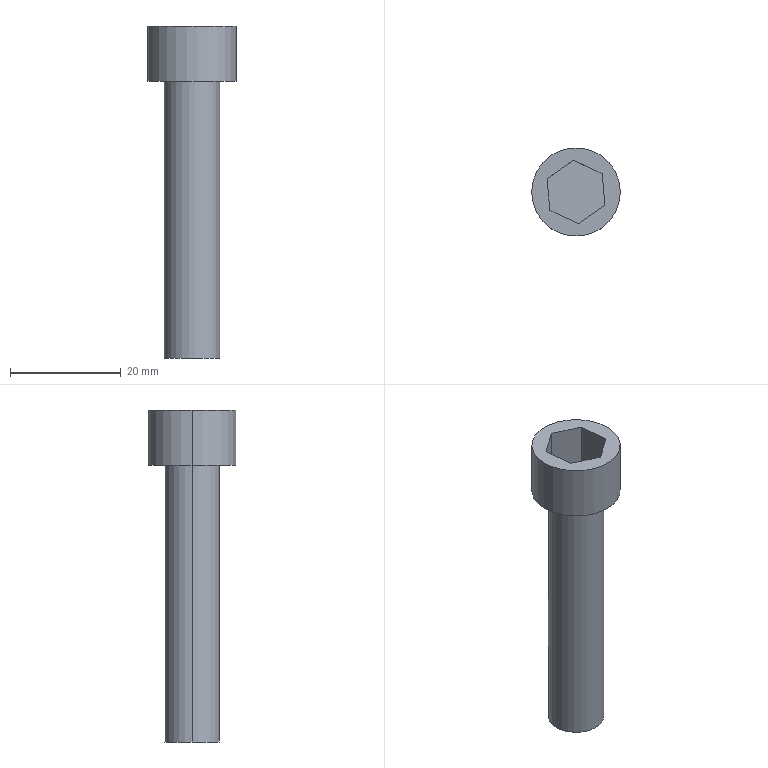Part | SolidWorks | features ICE 2, Extrusion 1 | 1 solid | 14 faces | box 16 x 16 x 60 mm | volume 5245 mm3 | plane 10 | cylinder 4 | commonest cylinder face diameters 10 x2 16 x2
STEP:
#1=CARTESIAN_POINT('',(8.,0.,60.));
#2=VERTEX_POINT('',#1);
#3=CARTESIAN_POINT('',(-8.,0.,60.));
#4=VERTEX_POINT('',#3);
#5=CARTESIAN_POINT('',(0.,0.,60.));
#6=DIRECTION('',(0.,0.,1.));
#7=DIRECTION('',(1.,0.,0.));
#8=AXIS2_PLACEMENT_3D('',#5,#6,#7);
#9=CIRCLE('',#8,8.);
#10=EDGE_CURVE('',#2,#4,#9,.T.);
#11=ORIENTED_EDGE('',*,*,#10,.F.);
#12=CARTESIAN_POINT('',(8.,0.,50.));
#13=VERTEX_POINT('',#12);
#14=CARTESIAN_POINT('',(8.,0.,60.));
#15=DIRECTION('',(0.,0.,-1.));
#16=VECTOR('',#15,1000.);
#17=LINE('',#14,#16);
#18=EDGE_CURVE('',#2,#13,#17,.T.);
#19=ORIENTED_EDGE('',*,*,#18,.T.);
#20=CARTESIAN_POINT('',(-8.,0.,50.));
#21=VERTEX_POINT('',#20);
#22=CARTESIAN_POINT('',(0.,0.,50.));
#23=DIRECTION('',(0.,0.,1.));
#24=DIRECTION('',(1.,0.,0.));
#25=AXIS2_PLACEMENT_3D('',#22,#23,#24);
#26=CIRCLE('',#25,8.);
#27=EDGE_CURVE('',#13,#21,#26,.T.);
#28=ORIENTED_EDGE('',*,*,#27,.T.);
#29=CARTESIAN_POINT('',(-8.,0.,60.));
#30=DIRECTION('',(0.,0.,-1.));
#31=VECTOR('',#30,1000.);
#32=LINE('',#29,#31);
#33=EDGE_CURVE('',#4,#21,#32,.T.);
#34=ORIENTED_EDGE('',*,*,#33,.F.);
#35=EDGE_LOOP('',(#11,#19,#28,#34));
#36=FACE_OUTER_BOUND('',#35,.T.);
#37=CARTESIAN_POINT('',(0.,0.,60.));
#38=DIRECTION('',(0.,0.,-1.));
#39=DIRECTION('',(-1.,0.,0.));
#40=AXIS2_PLACEMENT_3D('',#37,#38,#39);
#41=CYLINDRICAL_SURFACE('',#40,8.);
#42=ADVANCED_FACE('',(#36),#41,.T.);
#43=CARTESIAN_POINT('',(5.,0.,50.));
#44=VERTEX_POINT('',#43);
#45=CARTESIAN_POINT('',(-5.,0.,50.));
#46=VERTEX_POINT('',#45);
#47=CARTESIAN_POINT('',(0.,0.,50.));
#48=DIRECTION('',(0.,0.,1.));
#49=DIRECTION('',(1.,0.,0.));
#50=AXIS2_PLACEMENT_3D('',#47,#48,#49);
#51=CIRCLE('',#50,5.);
#52=EDGE_CURVE('',#44,#46,#51,.T.);
#53=ORIENTED_EDGE('',*,*,#52,.F.);
#54=CARTESIAN_POINT('',(5.,0.,0.));
#55=VERTEX_POINT('',#54);
#56=CARTESIAN_POINT('',(5.,0.,50.));
#57=DIRECTION('',(0.,0.,-1.));
#58=VECTOR('',#57,1000.);
#59=LINE('',#56,#58);
#60=EDGE_CURVE('',#44,#55,#59,.T.);
#61=ORIENTED_EDGE('',*,*,#60,.T.);
#62=CARTESIAN_POINT('',(-5.,0.,0.));
#63=VERTEX_POINT('',#62);
#64=CARTESIAN_POINT('',(0.,0.,0.));
#65=DIRECTION('',(0.,0.,1.));
#66=DIRECTION('',(1.,0.,0.));
#67=AXIS2_PLACEMENT_3D('',#64,#65,#66);
#68=CIRCLE('',#67,5.);
#69=EDGE_CURVE('',#55,#63,#68,.T.);
#70=ORIENTED_EDGE('',*,*,#69,.T.);
#71=CARTESIAN_POINT('',(-5.,0.,50.));
#72=DIRECTION('',(0.,0.,-1.));
#73=VECTOR('',#72,1000.);
#74=LINE('',#71,#73);
#75=EDGE_CURVE('',#46,#63,#74,.T.);
#76=ORIENTED_EDGE('',*,*,#75,.F.);
#77=EDGE_LOOP('',(#53,#61,#70,#76));
#78=FACE_OUTER_BOUND('',#77,.T.);
#79=CARTESIAN_POINT('',(0.,0.,50.));
#80=DIRECTION('',(0.,0.,-1.));
#81=DIRECTION('',(-1.,0.,0.));
#82=AXIS2_PLACEMENT_3D('',#79,#80,#81);
#83=CYLINDRICAL_SURFACE('',#82,5.);
#84=ADVANCED_FACE('',(#78),#83,.T.);
#85=ORIENTED_EDGE('',*,*,#60,.F.);
#86=CARTESIAN_POINT('',(0.,0.,50.));
#87=DIRECTION('',(0.,0.,1.));
#88=DIRECTION('',(1.,0.,0.));
#89=AXIS2_PLACEMENT_3D('',#86,#87,#88);
#90=CIRCLE('',#89,5.);
#91=EDGE_CURVE('',#46,#44,#90,.T.);
#92=ORIENTED_EDGE('',*,*,#91,.F.);
#93=ORIENTED_EDGE('',*,*,#75,.T.);
#94=CARTESIAN_POINT('',(0.,0.,0.));
#95=DIRECTION('',(0.,0.,1.));
#96=DIRECTION('',(1.,0.,0.));
#97=AXIS2_PLACEMENT_3D('',#94,#95,#96);
#98=CIRCLE('',#97,5.);
#99=EDGE_CURVE('',#63,#55,#98,.T.);
#100=ORIENTED_EDGE('',*,*,#99,.T.);
#101=EDGE_LOOP('',(#85,#92,#93,#100));
#102=FACE_OUTER_BOUND('',#101,.T.);
#103=CARTESIAN_POINT('',(0.,0.,50.));
#104=DIRECTION('',(0.,0.,-1.));
#105=DIRECTION('',(-1.,0.,0.));
#106=AXIS2_PLACEMENT_3D('',#103,#104,#105);
#107=CYLINDRICAL_SURFACE('',#106,5.);
#108=ADVANCED_FACE('',(#102),#107,.T.);
#109=ORIENTED_EDGE('',*,*,#99,.F.);
#110=ORIENTED_EDGE('',*,*,#69,.F.);
#111=EDGE_LOOP('',(#109,#110));
#112=FACE_OUTER_BOUND('',#111,.T.);
#113=CARTESIAN_POINT('',(0.,0.,0.));
#114=DIRECTION('',(0.,0.,1.));
#115=DIRECTION('',(1.,0.,0.));
#116=AXIS2_PLACEMENT_3D('',#113,#114,#115);
#117=PLANE('',#116);
#118=ADVANCED_FACE('',(#112),#117,.F.);
#119=ORIENTED_EDGE('',*,*,#18,.F.);
#120=CARTESIAN_POINT('',(0.,0.,60.));
#121=DIRECTION('',(0.,0.,1.));
#122=DIRECTION('',(1.,0.,0.));
#123=AXIS2_PLACEMENT_3D('',#120,#121,#122);
#124=CIRCLE('',#123,8.);
#125=EDGE_CURVE('',#4,#2,#124,.T.);
#126=ORIENTED_EDGE('',*,*,#125,.F.);
#127=ORIENTED_EDGE('',*,*,#33,.T.);
#128=CARTESIAN_POINT('',(0.,0.,50.));
#129=DIRECTION('',(0.,0.,1.));
#130=DIRECTION('',(1.,0.,0.));
#131=AXIS2_PLACEMENT_3D('',#128,#129,#130);
#132=CIRCLE('',#131,8.);
#133=EDGE_CURVE('',#21,#13,#132,.T.);
#134=ORIENTED_EDGE('',*,*,#133,.T.);
#135=EDGE_LOOP('',(#119,#126,#127,#134));
#136=FACE_OUTER_BOUND('',#135,.T.);
#137=CARTESIAN_POINT('',(0.,0.,60.));
#138=DIRECTION('',(0.,0.,-1.));
#139=DIRECTION('',(-1.,0.,0.));
#140=AXIS2_PLACEMENT_3D('',#137,#138,#139);
#141=CYLINDRICAL_SURFACE('',#140,8.);
#142=ADVANCED_FACE('',(#136),#141,.T.);
#143=CARTESIAN_POINT('',(-4.723,-3.321,60.));
#144=VERTEX_POINT('',#143);
#145=CARTESIAN_POINT('',(0.5141,-5.751,60.));
#146=VERTEX_POINT('',#145);
#147=CARTESIAN_POINT('',(-4.723,-3.321,60.));
#148=DIRECTION('',(0.9071,-0.4209,0.));
#149=VECTOR('',#148,1000.);
#150=LINE('',#147,#149);
#151=EDGE_CURVE('',#144,#146,#150,.T.);
#152=ORIENTED_EDGE('',*,*,#151,.F.);
#153=CARTESIAN_POINT('',(-5.237,2.43,60.));
#154=VERTEX_POINT('',#153);
#155=CARTESIAN_POINT('',(-5.237,2.43,60.));
#156=DIRECTION('',(0.08905,-0.996,0.));
#157=VECTOR('',#156,1000.);
#158=LINE('',#155,#157);
#159=EDGE_CURVE('',#154,#144,#158,.T.);
#160=ORIENTED_EDGE('',*,*,#159,.F.);
#161=CARTESIAN_POINT('',(-0.5141,5.751,60.));
#162=VERTEX_POINT('',#161);
#163=CARTESIAN_POINT('',(-0.5141,5.751,60.));
#164=DIRECTION('',(-0.8181,-0.5751,0.));
#165=VECTOR('',#164,1000.);
#166=LINE('',#163,#165);
#167=EDGE_CURVE('',#162,#154,#166,.T.);
#168=ORIENTED_EDGE('',*,*,#167,.F.);
#169=CARTESIAN_POINT('',(4.723,3.321,60.));
#170=VERTEX_POINT('',#169);
#171=CARTESIAN_POINT('',(4.723,3.321,60.));
#172=DIRECTION('',(-0.9071,0.4209,0.));
#173=VECTOR('',#172,1000.);
#174=LINE('',#171,#173);
#175=EDGE_CURVE('',#170,#162,#174,.T.);
#176=ORIENTED_EDGE('',*,*,#175,.F.);
#177=CARTESIAN_POINT('',(5.237,-2.43,60.));
#178=VERTEX_POINT('',#177);
#179=CARTESIAN_POINT('',(5.237,-2.43,60.));
#180=DIRECTION('',(-0.08905,0.996,0.));
#181=VECTOR('',#180,1000.);
#182=LINE('',#179,#181);
#183=EDGE_CURVE('',#178,#170,#182,.T.);
#184=ORIENTED_EDGE('',*,*,#183,.F.);
#185=CARTESIAN_POINT('',(0.5141,-5.751,60.));
#186=DIRECTION('',(0.8181,0.5751,0.));
#187=VECTOR('',#186,1000.);
#188=LINE('',#185,#187);
#189=EDGE_CURVE('',#146,#178,#188,.T.);
#190=ORIENTED_EDGE('',*,*,#189,.F.);
#191=EDGE_LOOP('',(#152,#160,#168,#176,#184,#190));
#192=FACE_BOUND('',#191,.T.);
#193=ORIENTED_EDGE('',*,*,#125,.T.);
#194=ORIENTED_EDGE('',*,*,#10,.T.);
#195=EDGE_LOOP('',(#193,#194));
#196=FACE_OUTER_BOUND('',#195,.T.);
#197=CARTESIAN_POINT('',(0.,0.,60.));
#198=DIRECTION('',(0.,0.,1.));
#199=DIRECTION('',(1.,0.,0.));
#200=AXIS2_PLACEMENT_3D('',#197,#198,#199);
#201=PLANE('',#200);
#202=ADVANCED_FACE('',(#192,#196),#201,.T.);
#203=ORIENTED_EDGE('',*,*,#91,.T.);
#204=ORIENTED_EDGE('',*,*,#52,.T.);
#205=EDGE_LOOP('',(#203,#204));
#206=FACE_BOUND('',#205,.T.);
#207=ORIENTED_EDGE('',*,*,#133,.F.);
#208=ORIENTED_EDGE('',*,*,#27,.F.);
#209=EDGE_LOOP('',(#207,#208));
#210=FACE_OUTER_BOUND('',#209,.T.);
#211=CARTESIAN_POINT('',(0.,0.,50.));
#212=DIRECTION('',(0.,0.,1.));
#213=DIRECTION('',(1.,0.,0.));
#214=AXIS2_PLACEMENT_3D('',#211,#212,#213);
#215=PLANE('',#214);
#216=ADVANCED_FACE('',(#206,#210),#215,.F.);
#217=ORIENTED_EDGE('',*,*,#151,.T.);
#218=CARTESIAN_POINT('',(0.5141,-5.751,52.));
#219=VERTEX_POINT('',#218);
#220=CARTESIAN_POINT('',(0.5141,-5.751,52.));
#221=DIRECTION('',(0.,0.,1.));
#222=VECTOR('',#221,1000.);
#223=LINE('',#220,#222);
#224=EDGE_CURVE('',#219,#146,#223,.T.);
#225=ORIENTED_EDGE('',*,*,#224,.F.);
#226=CARTESIAN_POINT('',(-4.723,-3.321,52.));
#227=VERTEX_POINT('',#226);
#228=CARTESIAN_POINT('',(-4.723,-3.321,52.));
#229=DIRECTION('',(0.9071,-0.4209,0.));
#230=VECTOR('',#229,1000.);
#231=LINE('',#228,#230);
#232=EDGE_CURVE('',#227,#219,#231,.T.);
#233=ORIENTED_EDGE('',*,*,#232,.F.);
#234=CARTESIAN_POINT('',(-4.723,-3.321,52.));
#235=DIRECTION('',(0.,0.,1.));
#236=VECTOR('',#235,1000.);
#237=LINE('',#234,#236);
#238=EDGE_CURVE('',#227,#144,#237,.T.);
#239=ORIENTED_EDGE('',*,*,#238,.T.);
#240=EDGE_LOOP('',(#217,#225,#233,#239));
#241=FACE_OUTER_BOUND('',#240,.T.);
#242=CARTESIAN_POINT('',(-4.723,-3.321,52.));
#243=DIRECTION('',(-0.4209,-0.9071,0.));
#244=DIRECTION('',(0.9071,-0.4209,0.));
#245=AXIS2_PLACEMENT_3D('',#242,#243,#244);
#246=PLANE('',#245);
#247=ADVANCED_FACE('',(#241),#246,.F.);
#248=ORIENTED_EDGE('',*,*,#159,.T.);
#249=ORIENTED_EDGE('',*,*,#238,.F.);
#250=CARTESIAN_POINT('',(-5.237,2.43,52.));
#251=VERTEX_POINT('',#250);
#252=CARTESIAN_POINT('',(-5.237,2.43,52.));
#253=DIRECTION('',(0.08905,-0.996,0.));
#254=VECTOR('',#253,1000.);
#255=LINE('',#252,#254);
#256=EDGE_CURVE('',#251,#227,#255,.T.);
#257=ORIENTED_EDGE('',*,*,#256,.F.);
#258=CARTESIAN_POINT('',(-5.237,2.43,52.));
#259=DIRECTION('',(0.,0.,1.));
#260=VECTOR('',#259,1000.);
#261=LINE('',#258,#260);
#262=EDGE_CURVE('',#251,#154,#261,.T.);
#263=ORIENTED_EDGE('',*,*,#262,.T.);
#264=EDGE_LOOP('',(#248,#249,#257,#263));
#265=FACE_OUTER_BOUND('',#264,.T.);
#266=CARTESIAN_POINT('',(-5.237,2.43,52.));
#267=DIRECTION('',(-0.996,-0.08905,0.));
#268=DIRECTION('',(0.08905,-0.996,0.));
#269=AXIS2_PLACEMENT_3D('',#266,#267,#268);
#270=PLANE('',#269);
#271=ADVANCED_FACE('',(#265),#270,.F.);
#272=ORIENTED_EDGE('',*,*,#167,.T.);
#273=ORIENTED_EDGE('',*,*,#262,.F.);
#274=CARTESIAN_POINT('',(-0.5141,5.751,52.));
#275=VERTEX_POINT('',#274);
#276=CARTESIAN_POINT('',(-0.5141,5.751,52.));
#277=DIRECTION('',(-0.8181,-0.5751,0.));
#278=VECTOR('',#277,1000.);
#279=LINE('',#276,#278);
#280=EDGE_CURVE('',#275,#251,#279,.T.);
#281=ORIENTED_EDGE('',*,*,#280,.F.);
#282=CARTESIAN_POINT('',(-0.5141,5.751,52.));
#283=DIRECTION('',(0.,0.,1.));
#284=VECTOR('',#283,1000.);
#285=LINE('',#282,#284);
#286=EDGE_CURVE('',#275,#162,#285,.T.);
#287=ORIENTED_EDGE('',*,*,#286,.T.);
#288=EDGE_LOOP('',(#272,#273,#281,#287));
#289=FACE_OUTER_BOUND('',#288,.T.);
#290=CARTESIAN_POINT('',(-0.5141,5.751,52.));
#291=DIRECTION('',(-0.5751,0.8181,0.));
#292=DIRECTION('',(-0.8181,-0.5751,0.));
#293=AXIS2_PLACEMENT_3D('',#290,#291,#292);
#294=PLANE('',#293);
#295=ADVANCED_FACE('',(#289),#294,.F.);
#296=ORIENTED_EDGE('',*,*,#175,.T.);
#297=ORIENTED_EDGE('',*,*,#286,.F.);
#298=CARTESIAN_POINT('',(4.723,3.321,52.));
#299=VERTEX_POINT('',#298);
#300=CARTESIAN_POINT('',(4.723,3.321,52.));
#301=DIRECTION('',(-0.9071,0.4209,0.));
#302=VECTOR('',#301,1000.);
#303=LINE('',#300,#302);
#304=EDGE_CURVE('',#299,#275,#303,.T.);
#305=ORIENTED_EDGE('',*,*,#304,.F.);
#306=CARTESIAN_POINT('',(4.723,3.321,52.));
#307=DIRECTION('',(0.,0.,1.));
#308=VECTOR('',#307,1000.);
#309=LINE('',#306,#308);
#310=EDGE_CURVE('',#299,#170,#309,.T.);
#311=ORIENTED_EDGE('',*,*,#310,.T.);
#312=EDGE_LOOP('',(#296,#297,#305,#311));
#313=FACE_OUTER_BOUND('',#312,.T.);
#314=CARTESIAN_POINT('',(4.723,3.321,52.));
#315=DIRECTION('',(0.4209,0.9071,0.));
#316=DIRECTION('',(-0.9071,0.4209,0.));
#317=AXIS2_PLACEMENT_3D('',#314,#315,#316);
#318=PLANE('',#317);
#319=ADVANCED_FACE('',(#313),#318,.F.);
#320=ORIENTED_EDGE('',*,*,#183,.T.);
#321=ORIENTED_EDGE('',*,*,#310,.F.);
#322=CARTESIAN_POINT('',(5.237,-2.43,52.));
#323=VERTEX_POINT('',#322);
#324=CARTESIAN_POINT('',(5.237,-2.43,52.));
#325=DIRECTION('',(-0.08905,0.996,0.));
#326=VECTOR('',#325,1000.);
#327=LINE('',#324,#326);
#328=EDGE_CURVE('',#323,#299,#327,.T.);
#329=ORIENTED_EDGE('',*,*,#328,.F.);
#330=CARTESIAN_POINT('',(5.237,-2.43,52.));
#331=DIRECTION('',(0.,0.,1.));
#332=VECTOR('',#331,1000.);
#333=LINE('',#330,#332);
#334=EDGE_CURVE('',#323,#178,#333,.T.);
#335=ORIENTED_EDGE('',*,*,#334,.T.);
#336=EDGE_LOOP('',(#320,#321,#329,#335));
#337=FACE_OUTER_BOUND('',#336,.T.);
#338=CARTESIAN_POINT('',(5.237,-2.43,52.));
#339=DIRECTION('',(0.996,0.08905,0.));
#340=DIRECTION('',(-0.08905,0.996,0.));
#341=AXIS2_PLACEMENT_3D('',#338,#339,#340);
#342=PLANE('',#341);
#343=ADVANCED_FACE('',(#337),#342,.F.);
#344=ORIENTED_EDGE('',*,*,#189,.T.);
#345=ORIENTED_EDGE('',*,*,#334,.F.);
#346=CARTESIAN_POINT('',(0.5141,-5.751,52.));
#347=DIRECTION('',(0.8181,0.5751,0.));
#348=VECTOR('',#347,1000.);
#349=LINE('',#346,#348);
#350=EDGE_CURVE('',#219,#323,#349,.T.);
#351=ORIENTED_EDGE('',*,*,#350,.F.);
#352=ORIENTED_EDGE('',*,*,#224,.T.);
#353=EDGE_LOOP('',(#344,#345,#351,#352));
#354=FACE_OUTER_BOUND('',#353,.T.);
#355=CARTESIAN_POINT('',(0.5141,-5.751,52.));
#356=DIRECTION('',(0.5751,-0.8181,0.));
#357=DIRECTION('',(0.8181,0.5751,0.));
#358=AXIS2_PLACEMENT_3D('',#355,#356,#357);
#359=PLANE('',#358);
#360=ADVANCED_FACE('',(#354),#359,.F.);
#361=ORIENTED_EDGE('',*,*,#232,.T.);
#362=ORIENTED_EDGE('',*,*,#350,.T.);
#363=ORIENTED_EDGE('',*,*,#328,.T.);
#364=ORIENTED_EDGE('',*,*,#304,.T.);
#365=ORIENTED_EDGE('',*,*,#280,.T.);
#366=ORIENTED_EDGE('',*,*,#256,.T.);
#367=EDGE_LOOP('',(#361,#362,#363,#364,#365,#366));
#368=FACE_OUTER_BOUND('',#367,.T.);
#369=CARTESIAN_POINT('',(0.,0.,52.));
#370=DIRECTION('',(0.,0.,1.));
#371=DIRECTION('',(1.,0.,0.));
#372=AXIS2_PLACEMENT_3D('',#369,#370,#371);
#373=PLANE('',#372);
#374=ADVANCED_FACE('',(#368),#373,.T.);
#375=CLOSED_SHELL('',(#42,#84,#108,#118,#142,#202,#216,#247,#271,#295,#319,#343,#360,#374));
#376=MANIFOLD_SOLID_BREP('',#375);
#377=CARTESIAN_POINT('',(0.,0.,0.));
#378=DIRECTION('',(0.,0.,1.));
#379=DIRECTION('',(1.,0.,0.));
#380=AXIS2_PLACEMENT_3D('',#377,#378,#379);
#381=(LENGTH_UNIT()NAMED_UNIT(*)SI_UNIT(.MILLI.,.METRE.));
#382=UNCERTAINTY_MEASURE_WITH_UNIT(LENGTH_MEASURE(0.00001),#381,'','');
#383=(NAMED_UNIT(*)PLANE_ANGLE_UNIT()SI_UNIT($,.RADIAN.));
#384=(NAMED_UNIT(*)SI_UNIT($,.STERADIAN.)SOLID_ANGLE_UNIT());
#385=(GEOMETRIC_REPRESENTATION_CONTEXT(3)GLOBAL_UNCERTAINTY_ASSIGNED_CONTEXT((#382))GLOBAL_UNIT_ASSIGNED_CONTEXT((#381,#383,#384))REPRESENTATION_CONTEXT('',''));
#386=ADVANCED_BREP_SHAPE_REPRESENTATION('',(#376,#380),#385);